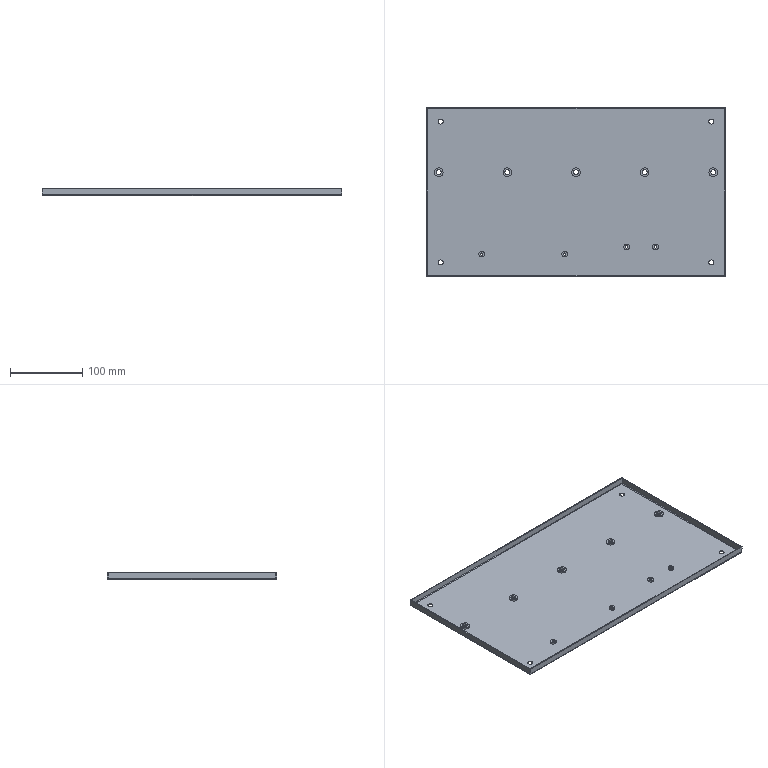Part | 1 solid | 91 faces | box 415 x 235 x 10 mm | volume 130458 mm3 | cylinder 52 | plane 31 | spline 8 | commonest cylinder face diameters 6.8 x10 12 x10 3.3 x8 7 x8 8 x8 1.473 x4